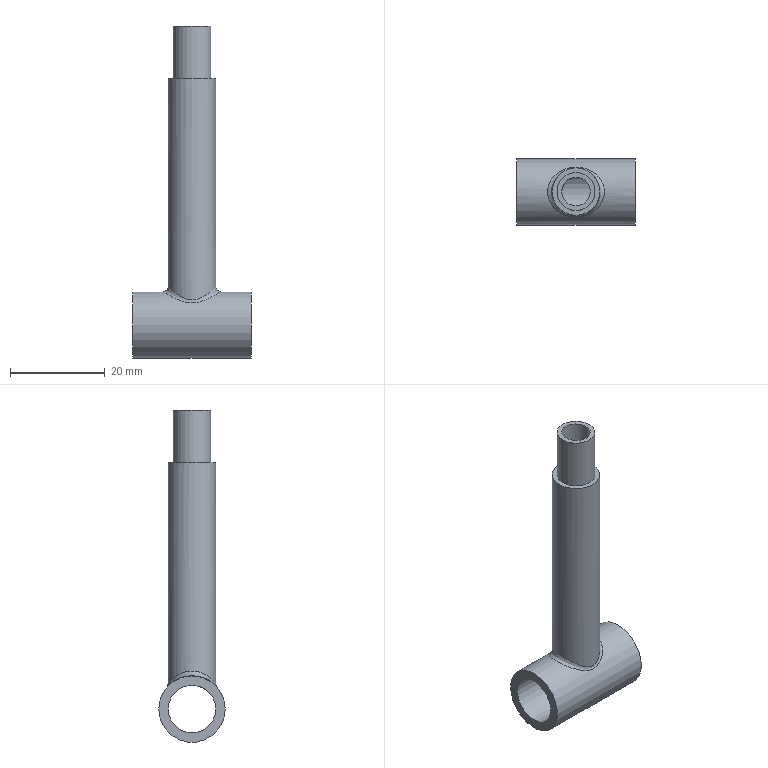Part | STEP file | 1-12.1 | 1 solid | 10 faces | box 25 x 14 x 70 mm | volume 4367 mm3 | cylinder 5 | plane 4 | spline 1 | commonest cylinder face diameters 10 x2 6 x1 8 x1 14 x1